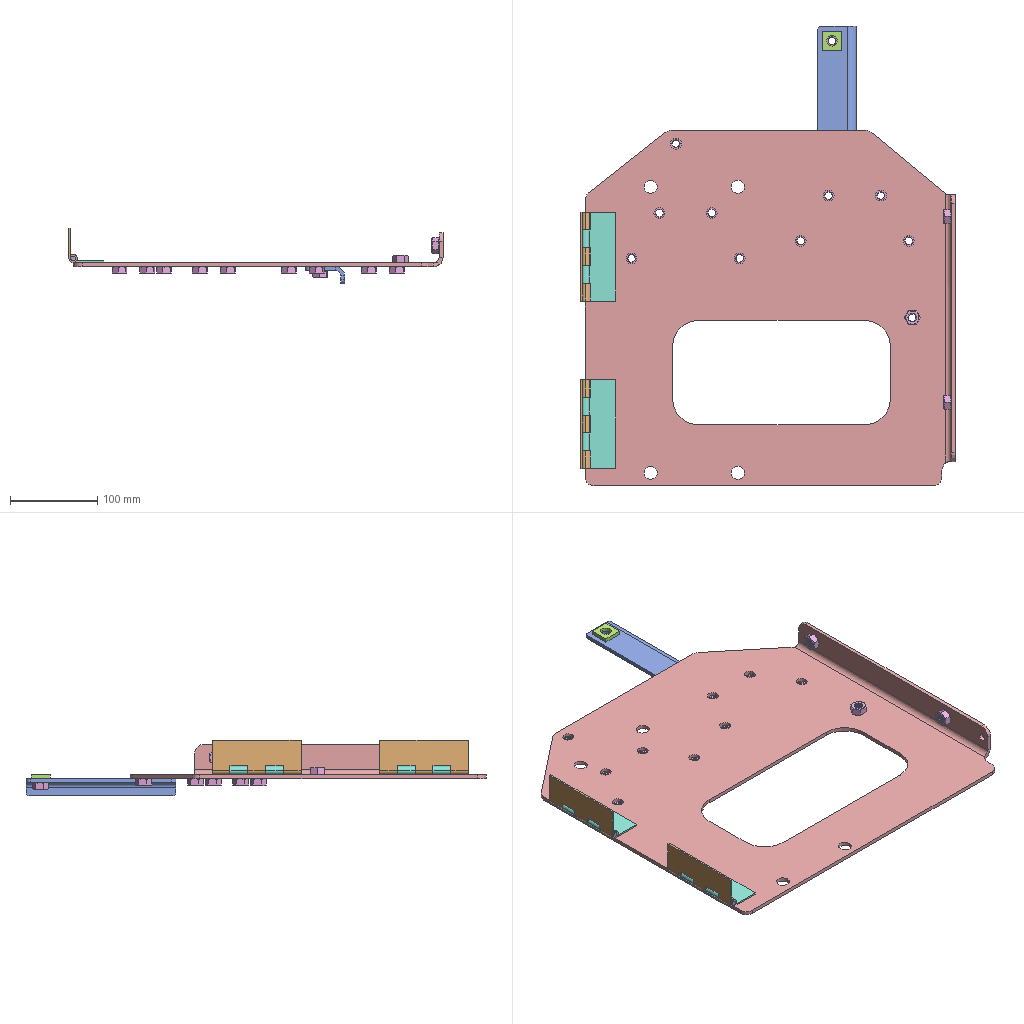Assembly | SolidWorks | 8 different items | 24 placed | box 429 x 528 x 64 mm
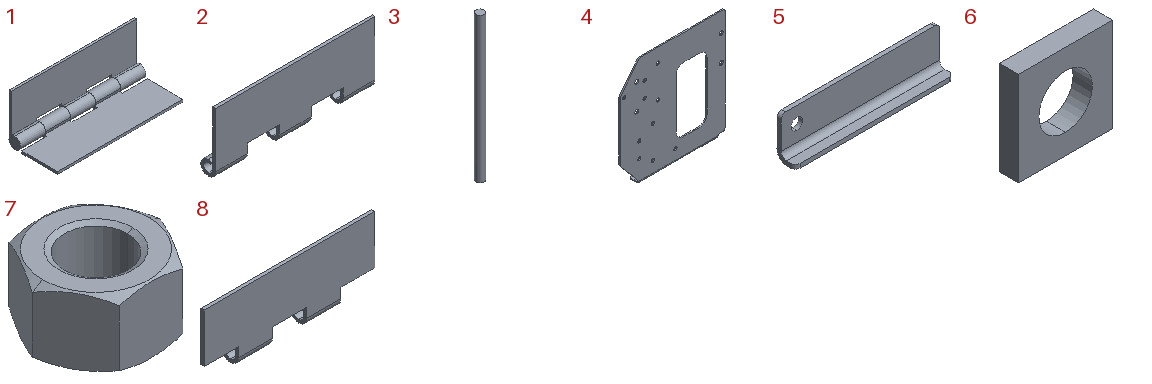Parts list (item | name | quantity | parent item | size | volume | features):
1 | (subassembly) | x2 | - | 102 x 39.7 x 39.7 mm | 18759 mm3 | -
2 | - | x2 | in 1 | 102 x 9.4 x 39.7 mm | 8617 mm3 | features FlatPattern 1, ICE 1, SMBaseFlange 1, SheetMetal 1
3 | - | x2 | in 1 | 5.6 x 5.6 x 102 mm | 2512 mm3 | features Extrusion 1
4 | - | x1 | - | 408 x 39 x 424 mm | 643319 mm3 | features ICE 3, Fillet 1, FlatPattern 1, SMBaseFlange 1, SheetMetal 1
5 | - | x1 | - | 172 x 20 x 45 mm | 43438 mm3 | features Fillet 1, FlatPattern 1, ICE 1, SMBaseFlange 1, SheetMetal 1
6 | - | x1 | - | 22 x 4.5 x 22 mm | 1626 mm3 | features FlatPattern 1, SMBaseFlange 1, SheetMetal 1
7 | - | x13 | - | 27.713 x 24 x 14.8 mm | 5071 mm3 | features RevCut 2, Chamfer 1, Extrusion 1, LPattern 1
8 | - | x2 | in 1 | 102 x 9.4 x 39.7 mm | 7631 mm3 | features FlatPattern 1, ICE 1, SMBaseFlange 1, SheetMetal 1
Mates (type | each side: item.copy, entity, surface, feature):
In the top assembly
Coincident | 4.1 face plane Base-Flange1 | 5.1 face plane Base-Flange1
Parallel | 4.1 face plane Base-Flange1 | 5.1 face plane Base-Flange1
DistanceDim | 5.1 face plane Base-Flange1 | 4.1 face cylinder Cut-Extrude1 | 2 times
Coincident | 5.1 face plane Base-Flange1 | 6.1 face plane Base-Flange1
Concentric | 5.1 face cylinder Cut-Extrude1 | 6.1 face cylinder Base-Flange1
Parallel | 5.1 face plane Base-Flange1 | 6.1 face plane Base-Flange1
Concentric | 4.1 face cylinder Cut-Extrude1 | 7.1 face cone EndChamfer
Coincident | 4.1 face plane Base-Flange1 | 7.1 face plane BaseNut
Concentric | 4.1 face cylinder Cut-Extrude3 | 7.2 face cone EndChamfer
Coincident | 4.1 face plane Base-Flange1 | 7.2 face plane BaseNut
Concentric | 4.1 face cylinder Cut-Extrude3 | 7.3 face cone EndChamfer
Coincident | 4.1 face plane Base-Flange1 | 7.3 face plane BaseNut
Concentric | 4.1 face cylinder Cut-Extrude1 | 7.4 face cone EndChamfer
Coincident | 4.1 face plane Base-Flange1 | 7.4 face plane BaseNut
Concentric | 4.1 face cylinder Cut-Extrude1 | 7.5 face cone EndChamfer
Coincident | 4.1 face plane Base-Flange1 | 7.5 face plane BaseNut
Concentric | 4.1 face cylinder Cut-Extrude1 | 7.6 face cone EndChamfer
Coincident | 4.1 face plane Base-Flange1 | 7.6 face plane BaseNut
Concentric | 4.1 face cylinder Cut-Extrude1 | 7.7 face cone EndChamfer
Coincident | 4.1 face plane Base-Flange1 | 7.7 face plane BaseNut
Concentric | 4.1 face cylinder Cut-Extrude1 | 7.8 face cone EndChamfer
Coincident | 4.1 face plane Base-Flange1 | 7.8 face plane BaseNut
Concentric | 4.1 face cylinder Cut-Extrude1 | 7.9 face cone EndChamfer
Coincident | 4.1 face plane Base-Flange1 | 7.9 face plane BaseNut
Concentric | 4.1 face cylinder Cut-Extrude1 | 7.10 face cone EndChamfer
Coincident | 4.1 face plane Base-Flange1 | 7.10 face plane BaseNut
Concentric | 4.1 face cylinder Cut-Extrude1 | 7.11 face cone EndChamfer
Coincident | 4.1 face plane Base-Flange1 | 7.11 face plane BaseNut
Concentric | 4.1 face cylinder Cut-Extrude1 | 7.12 face cone EndChamfer
Coincident | 4.1 face plane Base-Flange1 | 7.12 face plane BaseNut
Concentric | 5.1 face cylinder Cut-Extrude1 | 7.13 face cone EndChamfer
Coincident | 5.1 face plane Base-Flange1 | 7.13 face plane BaseNut
Coincident | 4.1 face plane Base-Flange1 | 8.1 face plane Base-Flange1
DistanceDim | 8.1 face plane Base-Flange1 | 4.1 face plane Base-Flange1
DistanceDim | 4.1 face plane Base-Flange1 | 2.1 face plane Base-Flange1
In subassembly 1
Concentric | 8.2 face cylinder Base bend 1 | 2.2 face cylinder Base bend 1
Coincident | 8.2 face plane Base-Flange1 | 2.2 face plane Base-Flange1
Perpendicular | 8.2 face plane Base-Flange1 | 2.2 face plane Base-Flange1
InPlace | 2.2 face plane Base-Flange1 | 3.1 plane